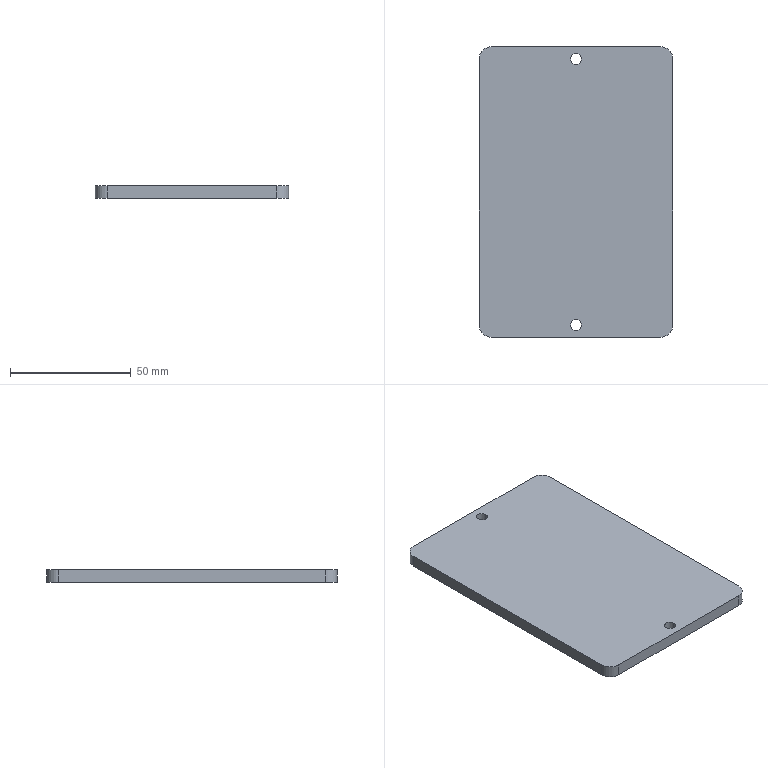Part | STEP file | Acrylic cover plate | 1 solid | 14 faces | box 80 x 120 x 5 mm | volume 47734 mm3 | cylinder 8 | plane 6 | commonest cylinder face diameters 4.5 x4 10 x4
STEP:
#1=CARTESIAN_POINT('',(0.,0.,0.));
#2=DIRECTION('',(0.,0.,1.));
#3=DIRECTION('',(1.,0.,0.));
#4=AXIS2_PLACEMENT_3D('',#1,#2,#3);
#5=CARTESIAN_POINT('',(-2.25,-55.,5.));
#6=VERTEX_POINT('',#5);
#7=CARTESIAN_POINT('',(-2.25,-55.,0.));
#8=VERTEX_POINT('',#7);
#9=CARTESIAN_POINT('',(-2.25,-55.,5.));
#10=DIRECTION('',(0.,0.,-1.));
#11=VECTOR('',#10,1.);
#12=LINE('',#9,#11);
#13=CARTESIAN_POINT('',(0.,-55.,5.));
#14=DIRECTION('',(0.,0.,-1.));
#15=DIRECTION('',(-1.,0.,0.));
#16=AXIS2_PLACEMENT_3D('',#13,#14,#15);
#17=CYLINDRICAL_SURFACE('',#16,2.25);
#18=CARTESIAN_POINT('',(6.283,0.));
#19=DIRECTION('',(0.,1.));
#20=VECTOR('',#19,1.);
#21=LINE('',#18,#20);
#22=(GEOMETRIC_REPRESENTATION_CONTEXT(2)PARAMETRIC_REPRESENTATION_CONTEXT()REPRESENTATION_CONTEXT('',''));
#23=DEFINITIONAL_REPRESENTATION('',(#21),#22);
#24=PCURVE('',#17,#23);
#25=CARTESIAN_POINT('',(0.,-55.,5.));
#26=DIRECTION('',(0.,0.,-1.));
#27=DIRECTION('',(-1.,0.,0.));
#28=AXIS2_PLACEMENT_3D('',#25,#26,#27);
#29=CYLINDRICAL_SURFACE('',#28,2.25);
#30=CARTESIAN_POINT('',(0.,0.));
#31=DIRECTION('',(0.,1.));
#32=VECTOR('',#31,1.);
#33=LINE('',#30,#32);
#34=(GEOMETRIC_REPRESENTATION_CONTEXT(2)PARAMETRIC_REPRESENTATION_CONTEXT()REPRESENTATION_CONTEXT('',''));
#35=DEFINITIONAL_REPRESENTATION('',(#33),#34);
#36=PCURVE('',#29,#35);
#37=SURFACE_CURVE('',#12,(#24,#36),.PCURVE_S1.);
#38=EDGE_CURVE('',#6,#8,#37,.T.);
#39=ORIENTED_EDGE('',*,*,#38,.T.);
#40=CARTESIAN_POINT('',(2.25,-55.,0.));
#41=VERTEX_POINT('',#40);
#42=CARTESIAN_POINT('',(0.,-55.,0.));
#43=DIRECTION('',(0.,0.,1.));
#44=DIRECTION('',(-1.,0.,0.));
#45=AXIS2_PLACEMENT_3D('',#42,#43,#44);
#46=CIRCLE('',#45,2.25);
#47=CARTESIAN_POINT('',(6.283,5.));
#48=DIRECTION('',(-1.,0.));
#49=VECTOR('',#48,1.);
#50=LINE('',#47,#49);
#51=(GEOMETRIC_REPRESENTATION_CONTEXT(2)PARAMETRIC_REPRESENTATION_CONTEXT()REPRESENTATION_CONTEXT('',''));
#52=DEFINITIONAL_REPRESENTATION('',(#50),#51);
#53=PCURVE('',#17,#52);
#54=CARTESIAN_POINT('',(35.,55.,0.));
#55=DIRECTION('',(0.,0.,-1.));
#56=DIRECTION('',(-1.,0.,0.));
#57=AXIS2_PLACEMENT_3D('',#54,#55,#56);
#58=PLANE('',#57);
#59=CARTESIAN_POINT('',(37.25,-110.));
#60=CARTESIAN_POINT('',(37.25,-113.897));
#61=CARTESIAN_POINT('',(33.875,-111.949));
#62=CARTESIAN_POINT('',(30.5,-110.));
#63=CARTESIAN_POINT('',(33.875,-108.051));
#64=CARTESIAN_POINT('',(37.25,-106.103));
#65=CARTESIAN_POINT('',(37.25,-110.));
#66=(BOUNDED_CURVE()B_SPLINE_CURVE(2,(#59,#60,#61,#62,#63,#64,#65),.UNSPECIFIED.,.T.,.F.)B_SPLINE_CURVE_WITH_KNOTS((1,2,2,2,2,1),(-2.094,0.,2.094,4.189,6.283,8.378),.UNSPECIFIED.)CURVE()GEOMETRIC_REPRESENTATION_ITEM()RATIONAL_B_SPLINE_CURVE((1.,0.5,1.,0.5,1.,0.5,1.))REPRESENTATION_ITEM(''));
#67=(GEOMETRIC_REPRESENTATION_CONTEXT(2)PARAMETRIC_REPRESENTATION_CONTEXT()REPRESENTATION_CONTEXT('',''));
#68=DEFINITIONAL_REPRESENTATION('',(#66),#67);
#69=PCURVE('',#58,#68);
#70=SURFACE_CURVE('',#46,(#53,#69),.PCURVE_S1.);
#71=EDGE_CURVE('',#8,#41,#70,.T.);
#72=ORIENTED_EDGE('',*,*,#71,.T.);
#73=CARTESIAN_POINT('',(2.25,-55.,5.));
#74=VERTEX_POINT('',#73);
#75=CARTESIAN_POINT('',(2.25,-55.,5.));
#76=DIRECTION('',(0.,0.,-1.));
#77=VECTOR('',#76,1.);
#78=LINE('',#75,#77);
#79=CARTESIAN_POINT('',(3.142,0.));
#80=DIRECTION('',(0.,1.));
#81=VECTOR('',#80,1.);
#82=LINE('',#79,#81);
#83=(GEOMETRIC_REPRESENTATION_CONTEXT(2)PARAMETRIC_REPRESENTATION_CONTEXT()REPRESENTATION_CONTEXT('',''));
#84=DEFINITIONAL_REPRESENTATION('',(#82),#83);
#85=PCURVE('',#17,#84);
#86=CARTESIAN_POINT('',(3.142,0.));
#87=DIRECTION('',(0.,1.));
#88=VECTOR('',#87,1.);
#89=LINE('',#86,#88);
#90=(GEOMETRIC_REPRESENTATION_CONTEXT(2)PARAMETRIC_REPRESENTATION_CONTEXT()REPRESENTATION_CONTEXT('',''));
#91=DEFINITIONAL_REPRESENTATION('',(#89),#90);
#92=PCURVE('',#29,#91);
#93=SURFACE_CURVE('',#78,(#85,#92),.PCURVE_S1.);
#94=EDGE_CURVE('',#74,#41,#93,.T.);
#95=ORIENTED_EDGE('',*,*,#94,.F.);
#96=CARTESIAN_POINT('',(0.,-55.,5.));
#97=DIRECTION('',(0.,0.,1.));
#98=DIRECTION('',(-1.,0.,0.));
#99=AXIS2_PLACEMENT_3D('',#96,#97,#98);
#100=CIRCLE('',#99,2.25);
#101=CARTESIAN_POINT('',(6.283,0.));
#102=DIRECTION('',(-1.,0.));
#103=VECTOR('',#102,1.);
#104=LINE('',#101,#103);
#105=(GEOMETRIC_REPRESENTATION_CONTEXT(2)PARAMETRIC_REPRESENTATION_CONTEXT()REPRESENTATION_CONTEXT('',''));
#106=DEFINITIONAL_REPRESENTATION('',(#104),#105);
#107=PCURVE('',#17,#106);
#108=CARTESIAN_POINT('',(35.,55.,5.));
#109=DIRECTION('',(0.,0.,-1.));
#110=DIRECTION('',(-1.,0.,0.));
#111=AXIS2_PLACEMENT_3D('',#108,#109,#110);
#112=PLANE('',#111);
#113=CARTESIAN_POINT('',(37.25,-110.));
#114=CARTESIAN_POINT('',(37.25,-113.897));
#115=CARTESIAN_POINT('',(33.875,-111.949));
#116=CARTESIAN_POINT('',(30.5,-110.));
#117=CARTESIAN_POINT('',(33.875,-108.051));
#118=CARTESIAN_POINT('',(37.25,-106.103));
#119=CARTESIAN_POINT('',(37.25,-110.));
#120=(BOUNDED_CURVE()B_SPLINE_CURVE(2,(#113,#114,#115,#116,#117,#118,#119),.UNSPECIFIED.,.T.,.F.)B_SPLINE_CURVE_WITH_KNOTS((1,2,2,2,2,1),(-2.094,0.,2.094,4.189,6.283,8.378),.UNSPECIFIED.)CURVE()GEOMETRIC_REPRESENTATION_ITEM()RATIONAL_B_SPLINE_CURVE((1.,0.5,1.,0.5,1.,0.5,1.))REPRESENTATION_ITEM(''));
#121=(GEOMETRIC_REPRESENTATION_CONTEXT(2)PARAMETRIC_REPRESENTATION_CONTEXT()REPRESENTATION_CONTEXT('',''));
#122=DEFINITIONAL_REPRESENTATION('',(#120),#121);
#123=PCURVE('',#112,#122);
#124=SURFACE_CURVE('',#100,(#107,#123),.PCURVE_S1.);
#125=EDGE_CURVE('',#6,#74,#124,.T.);
#126=ORIENTED_EDGE('',*,*,#125,.F.);
#127=EDGE_LOOP('',(#39,#72,#95,#126));
#128=FACE_BOUND('',#127,.F.);
#129=ADVANCED_FACE('',(#128),#17,.F.);
#130=CARTESIAN_POINT('',(-2.25,55.,5.));
#131=VERTEX_POINT('',#130);
#132=CARTESIAN_POINT('',(-2.25,55.,0.));
#133=VERTEX_POINT('',#132);
#134=CARTESIAN_POINT('',(-2.25,55.,5.));
#135=DIRECTION('',(0.,0.,-1.));
#136=VECTOR('',#135,1.);
#137=LINE('',#134,#136);
#138=CARTESIAN_POINT('',(0.,55.,5.));
#139=DIRECTION('',(0.,0.,-1.));
#140=DIRECTION('',(-1.,0.,0.));
#141=AXIS2_PLACEMENT_3D('',#138,#139,#140);
#142=CYLINDRICAL_SURFACE('',#141,2.25);
#143=CARTESIAN_POINT('',(6.283,0.));
#144=DIRECTION('',(0.,1.));
#145=VECTOR('',#144,1.);
#146=LINE('',#143,#145);
#147=(GEOMETRIC_REPRESENTATION_CONTEXT(2)PARAMETRIC_REPRESENTATION_CONTEXT()REPRESENTATION_CONTEXT('',''));
#148=DEFINITIONAL_REPRESENTATION('',(#146),#147);
#149=PCURVE('',#142,#148);
#150=CARTESIAN_POINT('',(0.,55.,5.));
#151=DIRECTION('',(0.,0.,-1.));
#152=DIRECTION('',(-1.,0.,0.));
#153=AXIS2_PLACEMENT_3D('',#150,#151,#152);
#154=CYLINDRICAL_SURFACE('',#153,2.25);
#155=CARTESIAN_POINT('',(0.,0.));
#156=DIRECTION('',(0.,1.));
#157=VECTOR('',#156,1.);
#158=LINE('',#155,#157);
#159=(GEOMETRIC_REPRESENTATION_CONTEXT(2)PARAMETRIC_REPRESENTATION_CONTEXT()REPRESENTATION_CONTEXT('',''));
#160=DEFINITIONAL_REPRESENTATION('',(#158),#159);
#161=PCURVE('',#154,#160);
#162=SURFACE_CURVE('',#137,(#149,#161),.PCURVE_S1.);
#163=EDGE_CURVE('',#131,#133,#162,.T.);
#164=ORIENTED_EDGE('',*,*,#163,.T.);
#165=CARTESIAN_POINT('',(2.25,55.,0.));
#166=VERTEX_POINT('',#165);
#167=CARTESIAN_POINT('',(0.,55.,0.));
#168=DIRECTION('',(0.,0.,1.));
#169=DIRECTION('',(-1.,0.,0.));
#170=AXIS2_PLACEMENT_3D('',#167,#168,#169);
#171=CIRCLE('',#170,2.25);
#172=CARTESIAN_POINT('',(6.283,5.));
#173=DIRECTION('',(-1.,0.));
#174=VECTOR('',#173,1.);
#175=LINE('',#172,#174);
#176=(GEOMETRIC_REPRESENTATION_CONTEXT(2)PARAMETRIC_REPRESENTATION_CONTEXT()REPRESENTATION_CONTEXT('',''));
#177=DEFINITIONAL_REPRESENTATION('',(#175),#176);
#178=PCURVE('',#142,#177);
#179=CARTESIAN_POINT('',(37.25,0.));
#180=CARTESIAN_POINT('',(37.25,-3.897));
#181=CARTESIAN_POINT('',(33.875,-1.949));
#182=CARTESIAN_POINT('',(30.5,0.));
#183=CARTESIAN_POINT('',(33.875,1.949));
#184=CARTESIAN_POINT('',(37.25,3.897));
#185=CARTESIAN_POINT('',(37.25,0.));
#186=(BOUNDED_CURVE()B_SPLINE_CURVE(2,(#179,#180,#181,#182,#183,#184,#185),.UNSPECIFIED.,.T.,.F.)B_SPLINE_CURVE_WITH_KNOTS((1,2,2,2,2,1),(-2.094,0.,2.094,4.189,6.283,8.378),.UNSPECIFIED.)CURVE()GEOMETRIC_REPRESENTATION_ITEM()RATIONAL_B_SPLINE_CURVE((1.,0.5,1.,0.5,1.,0.5,1.))REPRESENTATION_ITEM(''));
#187=(GEOMETRIC_REPRESENTATION_CONTEXT(2)PARAMETRIC_REPRESENTATION_CONTEXT()REPRESENTATION_CONTEXT('',''));
#188=DEFINITIONAL_REPRESENTATION('',(#186),#187);
#189=PCURVE('',#58,#188);
#190=SURFACE_CURVE('',#171,(#178,#189),.PCURVE_S1.);
#191=EDGE_CURVE('',#133,#166,#190,.T.);
#192=ORIENTED_EDGE('',*,*,#191,.T.);
#193=CARTESIAN_POINT('',(2.25,55.,5.));
#194=VERTEX_POINT('',#193);
#195=CARTESIAN_POINT('',(2.25,55.,5.));
#196=DIRECTION('',(0.,0.,-1.));
#197=VECTOR('',#196,1.);
#198=LINE('',#195,#197);
#199=CARTESIAN_POINT('',(3.142,0.));
#200=DIRECTION('',(0.,1.));
#201=VECTOR('',#200,1.);
#202=LINE('',#199,#201);
#203=(GEOMETRIC_REPRESENTATION_CONTEXT(2)PARAMETRIC_REPRESENTATION_CONTEXT()REPRESENTATION_CONTEXT('',''));
#204=DEFINITIONAL_REPRESENTATION('',(#202),#203);
#205=PCURVE('',#142,#204);
#206=CARTESIAN_POINT('',(3.142,0.));
#207=DIRECTION('',(0.,1.));
#208=VECTOR('',#207,1.);
#209=LINE('',#206,#208);
#210=(GEOMETRIC_REPRESENTATION_CONTEXT(2)PARAMETRIC_REPRESENTATION_CONTEXT()REPRESENTATION_CONTEXT('',''));
#211=DEFINITIONAL_REPRESENTATION('',(#209),#210);
#212=PCURVE('',#154,#211);
#213=SURFACE_CURVE('',#198,(#205,#212),.PCURVE_S1.);
#214=EDGE_CURVE('',#194,#166,#213,.T.);
#215=ORIENTED_EDGE('',*,*,#214,.F.);
#216=CARTESIAN_POINT('',(0.,55.,5.));
#217=DIRECTION('',(0.,0.,1.));
#218=DIRECTION('',(-1.,0.,0.));
#219=AXIS2_PLACEMENT_3D('',#216,#217,#218);
#220=CIRCLE('',#219,2.25);
#221=CARTESIAN_POINT('',(6.283,0.));
#222=DIRECTION('',(-1.,0.));
#223=VECTOR('',#222,1.);
#224=LINE('',#221,#223);
#225=(GEOMETRIC_REPRESENTATION_CONTEXT(2)PARAMETRIC_REPRESENTATION_CONTEXT()REPRESENTATION_CONTEXT('',''));
#226=DEFINITIONAL_REPRESENTATION('',(#224),#225);
#227=PCURVE('',#142,#226);
#228=CARTESIAN_POINT('',(37.25,0.));
#229=CARTESIAN_POINT('',(37.25,-3.897));
#230=CARTESIAN_POINT('',(33.875,-1.949));
#231=CARTESIAN_POINT('',(30.5,0.));
#232=CARTESIAN_POINT('',(33.875,1.949));
#233=CARTESIAN_POINT('',(37.25,3.897));
#234=CARTESIAN_POINT('',(37.25,0.));
#235=(BOUNDED_CURVE()B_SPLINE_CURVE(2,(#228,#229,#230,#231,#232,#233,#234),.UNSPECIFIED.,.T.,.F.)B_SPLINE_CURVE_WITH_KNOTS((1,2,2,2,2,1),(-2.094,0.,2.094,4.189,6.283,8.378),.UNSPECIFIED.)CURVE()GEOMETRIC_REPRESENTATION_ITEM()RATIONAL_B_SPLINE_CURVE((1.,0.5,1.,0.5,1.,0.5,1.))REPRESENTATION_ITEM(''));
#236=(GEOMETRIC_REPRESENTATION_CONTEXT(2)PARAMETRIC_REPRESENTATION_CONTEXT()REPRESENTATION_CONTEXT('',''));
#237=DEFINITIONAL_REPRESENTATION('',(#235),#236);
#238=PCURVE('',#112,#237);
#239=SURFACE_CURVE('',#220,(#227,#238),.PCURVE_S1.);
#240=EDGE_CURVE('',#131,#194,#239,.T.);
#241=ORIENTED_EDGE('',*,*,#240,.F.);
#242=EDGE_LOOP('',(#164,#192,#215,#241));
#243=FACE_BOUND('',#242,.F.);
#244=ADVANCED_FACE('',(#243),#142,.F.);
#245=ORIENTED_EDGE('',*,*,#125,.F.);
#246=CARTESIAN_POINT('',(0.,-55.,5.));
#247=DIRECTION('',(0.,0.,1.));
#248=DIRECTION('',(-1.,0.,0.));
#249=AXIS2_PLACEMENT_3D('',#246,#247,#248);
#250=CIRCLE('',#249,2.25);
#251=CARTESIAN_POINT('',(37.25,-110.));
#252=CARTESIAN_POINT('',(37.25,-113.897));
#253=CARTESIAN_POINT('',(33.875,-111.949));
#254=CARTESIAN_POINT('',(30.5,-110.));
#255=CARTESIAN_POINT('',(33.875,-108.051));
#256=CARTESIAN_POINT('',(37.25,-106.103));
#257=CARTESIAN_POINT('',(37.25,-110.));
#258=(BOUNDED_CURVE()B_SPLINE_CURVE(2,(#251,#252,#253,#254,#255,#256,#257),.UNSPECIFIED.,.T.,.F.)B_SPLINE_CURVE_WITH_KNOTS((1,2,2,2,2,1),(-2.094,0.,2.094,4.189,6.283,8.378),.UNSPECIFIED.)CURVE()GEOMETRIC_REPRESENTATION_ITEM()RATIONAL_B_SPLINE_CURVE((1.,0.5,1.,0.5,1.,0.5,1.))REPRESENTATION_ITEM(''));
#259=(GEOMETRIC_REPRESENTATION_CONTEXT(2)PARAMETRIC_REPRESENTATION_CONTEXT()REPRESENTATION_CONTEXT('',''));
#260=DEFINITIONAL_REPRESENTATION('',(#258),#259);
#261=PCURVE('',#112,#260);
#262=CARTESIAN_POINT('',(6.283,0.));
#263=DIRECTION('',(-1.,0.));
#264=VECTOR('',#263,1.);
#265=LINE('',#262,#264);
#266=(GEOMETRIC_REPRESENTATION_CONTEXT(2)PARAMETRIC_REPRESENTATION_CONTEXT()REPRESENTATION_CONTEXT('',''));
#267=DEFINITIONAL_REPRESENTATION('',(#265),#266);
#268=PCURVE('',#29,#267);
#269=SURFACE_CURVE('',#250,(#261,#268),.PCURVE_S1.);
#270=EDGE_CURVE('',#74,#6,#269,.T.);
#271=ORIENTED_EDGE('',*,*,#270,.F.);
#272=EDGE_LOOP('',(#245,#271));
#273=FACE_BOUND('',#272,.T.);
#274=CARTESIAN_POINT('',(-35.,60.,5.));
#275=VERTEX_POINT('',#274);
#276=CARTESIAN_POINT('',(35.,60.,5.));
#277=VERTEX_POINT('',#276);
#278=CARTESIAN_POINT('',(35.,60.,5.));
#279=DIRECTION('',(1.,0.,0.));
#280=VECTOR('',#279,1.);
#281=LINE('',#278,#280);
#282=CARTESIAN_POINT('',(0.,5.));
#283=DIRECTION('',(-1.,0.));
#284=VECTOR('',#283,1.);
#285=LINE('',#282,#284);
#286=(GEOMETRIC_REPRESENTATION_CONTEXT(2)PARAMETRIC_REPRESENTATION_CONTEXT()REPRESENTATION_CONTEXT('',''));
#287=DEFINITIONAL_REPRESENTATION('',(#285),#286);
#288=PCURVE('',#112,#287);
#289=CARTESIAN_POINT('',(-35.,60.,5.));
#290=DIRECTION('',(0.,-1.,0.));
#291=DIRECTION('',(0.,0.,-1.));
#292=AXIS2_PLACEMENT_3D('',#289,#290,#291);
#293=PLANE('',#292);
#294=CARTESIAN_POINT('',(0.,70.));
#295=DIRECTION('',(0.,1.));
#296=VECTOR('',#295,1.);
#297=LINE('',#294,#296);
#298=(GEOMETRIC_REPRESENTATION_CONTEXT(2)PARAMETRIC_REPRESENTATION_CONTEXT()REPRESENTATION_CONTEXT('',''));
#299=DEFINITIONAL_REPRESENTATION('',(#297),#298);
#300=PCURVE('',#293,#299);
#301=SURFACE_CURVE('',#281,(#288,#300),.PCURVE_S1.);
#302=EDGE_CURVE('',#275,#277,#301,.T.);
#303=ORIENTED_EDGE('',*,*,#302,.F.);
#304=CARTESIAN_POINT('',(-40.,55.,5.));
#305=VERTEX_POINT('',#304);
#306=CARTESIAN_POINT('',(-35.,55.,5.));
#307=DIRECTION('',(0.,0.,-1.));
#308=DIRECTION('',(-1.,0.,0.));
#309=AXIS2_PLACEMENT_3D('',#306,#307,#308);
#310=CIRCLE('',#309,5.);
#311=CARTESIAN_POINT('',(70.,0.));
#312=DIRECTION('',(1.,0.));
#313=AXIS2_PLACEMENT_2D('',#311,#312);
#314=CIRCLE('',#313,5.);
#315=(GEOMETRIC_REPRESENTATION_CONTEXT(2)PARAMETRIC_REPRESENTATION_CONTEXT()REPRESENTATION_CONTEXT('',''));
#316=DEFINITIONAL_REPRESENTATION('',(#314),#315);
#317=PCURVE('',#112,#316);
#318=CARTESIAN_POINT('',(-35.,55.,5.));
#319=DIRECTION('',(0.,0.,-1.));
#320=DIRECTION('',(-1.,0.,0.));
#321=AXIS2_PLACEMENT_3D('',#318,#319,#320);
#322=CYLINDRICAL_SURFACE('',#321,5.);
#323=CARTESIAN_POINT('',(0.,0.));
#324=DIRECTION('',(1.,0.));
#325=VECTOR('',#324,1.);
#326=LINE('',#323,#325);
#327=(GEOMETRIC_REPRESENTATION_CONTEXT(2)PARAMETRIC_REPRESENTATION_CONTEXT()REPRESENTATION_CONTEXT('',''));
#328=DEFINITIONAL_REPRESENTATION('',(#326),#327);
#329=PCURVE('',#322,#328);
#330=SURFACE_CURVE('',#310,(#317,#329),.PCURVE_S1.);
#331=EDGE_CURVE('',#305,#275,#330,.T.);
#332=ORIENTED_EDGE('',*,*,#331,.F.);
#333=CARTESIAN_POINT('',(-40.,-55.,5.));
#334=VERTEX_POINT('',#333);
#335=CARTESIAN_POINT('',(-40.,55.,5.));
#336=DIRECTION('',(0.,1.,0.));
#337=VECTOR('',#336,1.);
#338=LINE('',#335,#337);
#339=CARTESIAN_POINT('',(75.,0.));
#340=DIRECTION('',(0.,1.));
#341=VECTOR('',#340,1.);
#342=LINE('',#339,#341);
#343=(GEOMETRIC_REPRESENTATION_CONTEXT(2)PARAMETRIC_REPRESENTATION_CONTEXT()REPRESENTATION_CONTEXT('',''));
#344=DEFINITIONAL_REPRESENTATION('',(#342),#343);
#345=PCURVE('',#112,#344);
#346=CARTESIAN_POINT('',(-40.,55.,5.));
#347=DIRECTION('',(1.,0.,0.));
#348=DIRECTION('',(0.,1.,0.));
#349=AXIS2_PLACEMENT_3D('',#346,#347,#348);
#350=PLANE('',#349);
#351=CARTESIAN_POINT('',(0.,0.));
#352=DIRECTION('',(1.,0.));
#353=VECTOR('',#352,1.);
#354=LINE('',#351,#353);
#355=(GEOMETRIC_REPRESENTATION_CONTEXT(2)PARAMETRIC_REPRESENTATION_CONTEXT()REPRESENTATION_CONTEXT('',''));
#356=DEFINITIONAL_REPRESENTATION('',(#354),#355);
#357=PCURVE('',#350,#356);
#358=SURFACE_CURVE('',#338,(#345,#357),.PCURVE_S1.);
#359=EDGE_CURVE('',#334,#305,#358,.T.);
#360=ORIENTED_EDGE('',*,*,#359,.F.);
#361=CARTESIAN_POINT('',(-35.,-60.,5.));
#362=VERTEX_POINT('',#361);
#363=CARTESIAN_POINT('',(-35.,-55.,5.));
#364=DIRECTION('',(0.,0.,-1.));
#365=DIRECTION('',(-1.,0.,0.));
#366=AXIS2_PLACEMENT_3D('',#363,#364,#365);
#367=CIRCLE('',#366,5.);
#368=CARTESIAN_POINT('',(70.,-110.));
#369=DIRECTION('',(1.,0.));
#370=AXIS2_PLACEMENT_2D('',#368,#369);
#371=CIRCLE('',#370,5.);
#372=(GEOMETRIC_REPRESENTATION_CONTEXT(2)PARAMETRIC_REPRESENTATION_CONTEXT()REPRESENTATION_CONTEXT('',''));
#373=DEFINITIONAL_REPRESENTATION('',(#371),#372);
#374=PCURVE('',#112,#373);
#375=CARTESIAN_POINT('',(-35.,-55.,5.));
#376=DIRECTION('',(0.,0.,-1.));
#377=DIRECTION('',(-1.,0.,0.));
#378=AXIS2_PLACEMENT_3D('',#375,#376,#377);
#379=CYLINDRICAL_SURFACE('',#378,5.);
#380=CARTESIAN_POINT('',(0.,0.));
#381=DIRECTION('',(1.,0.));
#382=VECTOR('',#381,1.);
#383=LINE('',#380,#382);
#384=(GEOMETRIC_REPRESENTATION_CONTEXT(2)PARAMETRIC_REPRESENTATION_CONTEXT()REPRESENTATION_CONTEXT('',''));
#385=DEFINITIONAL_REPRESENTATION('',(#383),#384);
#386=PCURVE('',#379,#385);
#387=SURFACE_CURVE('',#367,(#374,#386),.PCURVE_S1.);
#388=EDGE_CURVE('',#362,#334,#387,.T.);
#389=ORIENTED_EDGE('',*,*,#388,.F.);
#390=CARTESIAN_POINT('',(35.,-60.,5.));
#391=VERTEX_POINT('',#390);
#392=CARTESIAN_POINT('',(35.,-60.,5.));
#393=DIRECTION('',(-1.,0.,0.));
#394=VECTOR('',#393,1.);
#395=LINE('',#392,#394);
#396=CARTESIAN_POINT('',(0.,-115.));
#397=DIRECTION('',(1.,0.));
#398=VECTOR('',#397,1.);
#399=LINE('',#396,#398);
#400=(GEOMETRIC_REPRESENTATION_CONTEXT(2)PARAMETRIC_REPRESENTATION_CONTEXT()REPRESENTATION_CONTEXT('',''));
#401=DEFINITIONAL_REPRESENTATION('',(#399),#400);
#402=PCURVE('',#112,#401);
#403=CARTESIAN_POINT('',(-35.,-60.,5.));
#404=DIRECTION('',(0.,1.,0.));
#405=DIRECTION('',(0.,0.,1.));
#406=AXIS2_PLACEMENT_3D('',#403,#404,#405);
#407=PLANE('',#406);
#408=CARTESIAN_POINT('',(0.,70.));
#409=DIRECTION('',(0.,-1.));
#410=VECTOR('',#409,1.);
#411=LINE('',#408,#410);
#412=(GEOMETRIC_REPRESENTATION_CONTEXT(2)PARAMETRIC_REPRESENTATION_CONTEXT()REPRESENTATION_CONTEXT('',''));
#413=DEFINITIONAL_REPRESENTATION('',(#411),#412);
#414=PCURVE('',#407,#413);
#415=SURFACE_CURVE('',#395,(#402,#414),.PCURVE_S1.);
#416=EDGE_CURVE('',#391,#362,#415,.T.);
#417=ORIENTED_EDGE('',*,*,#416,.F.);
#418=CARTESIAN_POINT('',(40.,-55.,5.));
#419=VERTEX_POINT('',#418);
#420=CARTESIAN_POINT('',(35.,-55.,5.));
#421=DIRECTION('',(0.,0.,-1.));
#422=DIRECTION('',(-1.,0.,0.));
#423=AXIS2_PLACEMENT_3D('',#420,#421,#422);
#424=CIRCLE('',#423,5.);
#425=CARTESIAN_POINT('',(0.,-110.));
#426=DIRECTION('',(1.,0.));
#427=AXIS2_PLACEMENT_2D('',#425,#426);
#428=CIRCLE('',#427,5.);
#429=(GEOMETRIC_REPRESENTATION_CONTEXT(2)PARAMETRIC_REPRESENTATION_CONTEXT()REPRESENTATION_CONTEXT('',''));
#430=DEFINITIONAL_REPRESENTATION('',(#428),#429);
#431=PCURVE('',#112,#430);
#432=CARTESIAN_POINT('',(35.,-55.,5.));
#433=DIRECTION('',(0.,0.,-1.));
#434=DIRECTION('',(-1.,0.,0.));
#435=AXIS2_PLACEMENT_3D('',#432,#433,#434);
#436=CYLINDRICAL_SURFACE('',#435,5.);
#437=CARTESIAN_POINT('',(0.,0.));
#438=DIRECTION('',(1.,0.));
#439=VECTOR('',#438,1.);
#440=LINE('',#437,#439);
#441=(GEOMETRIC_REPRESENTATION_CONTEXT(2)PARAMETRIC_REPRESENTATION_CONTEXT()REPRESENTATION_CONTEXT('',''));
#442=DEFINITIONAL_REPRESENTATION('',(#440),#441);
#443=PCURVE('',#436,#442);
#444=SURFACE_CURVE('',#424,(#431,#443),.PCURVE_S1.);
#445=EDGE_CURVE('',#419,#391,#444,.T.);
#446=ORIENTED_EDGE('',*,*,#445,.F.);
#447=CARTESIAN_POINT('',(40.,55.,5.));
#448=VERTEX_POINT('',#447);
#449=CARTESIAN_POINT('',(40.,55.,5.));
#450=DIRECTION('',(0.,-1.,0.));
#451=VECTOR('',#450,1.);
#452=LINE('',#449,#451);
#453=CARTESIAN_POINT('',(-5.,0.));
#454=DIRECTION('',(0.,-1.));
#455=VECTOR('',#454,1.);
#456=LINE('',#453,#455);
#457=(GEOMETRIC_REPRESENTATION_CONTEXT(2)PARAMETRIC_REPRESENTATION_CONTEXT()REPRESENTATION_CONTEXT('',''));
#458=DEFINITIONAL_REPRESENTATION('',(#456),#457);
#459=PCURVE('',#112,#458);
#460=CARTESIAN_POINT('',(40.,55.,5.));
#461=DIRECTION('',(-1.,0.,0.));
#462=DIRECTION('',(0.,-1.,0.));
#463=AXIS2_PLACEMENT_3D('',#460,#461,#462);
#464=PLANE('',#463);
#465=CARTESIAN_POINT('',(0.,0.));
#466=DIRECTION('',(1.,0.));
#467=VECTOR('',#466,1.);
#468=LINE('',#465,#467);
#469=(GEOMETRIC_REPRESENTATION_CONTEXT(2)PARAMETRIC_REPRESENTATION_CONTEXT()REPRESENTATION_CONTEXT('',''));
#470=DEFINITIONAL_REPRESENTATION('',(#468),#469);
#471=PCURVE('',#464,#470);
#472=SURFACE_CURVE('',#452,(#459,#471),.PCURVE_S1.);
#473=EDGE_CURVE('',#448,#419,#472,.T.);
#474=ORIENTED_EDGE('',*,*,#473,.F.);
#475=CARTESIAN_POINT('',(35.,55.,5.));
#476=DIRECTION('',(0.,0.,-1.));
#477=DIRECTION('',(-1.,0.,0.));
#478=AXIS2_PLACEMENT_3D('',#475,#476,#477);
#479=CIRCLE('',#478,5.);
#480=CARTESIAN_POINT('',(0.,0.));
#481=DIRECTION('',(1.,0.));
#482=AXIS2_PLACEMENT_2D('',#480,#481);
#483=CIRCLE('',#482,5.);
#484=(GEOMETRIC_REPRESENTATION_CONTEXT(2)PARAMETRIC_REPRESENTATION_CONTEXT()REPRESENTATION_CONTEXT('',''));
#485=DEFINITIONAL_REPRESENTATION('',(#483),#484);
#486=PCURVE('',#112,#485);
#487=CARTESIAN_POINT('',(35.,55.,5.));
#488=DIRECTION('',(0.,0.,-1.));
#489=DIRECTION('',(-1.,0.,0.));
#490=AXIS2_PLACEMENT_3D('',#487,#488,#489);
#491=CYLINDRICAL_SURFACE('',#490,5.);
#492=CARTESIAN_POINT('',(0.,0.));
#493=DIRECTION('',(1.,0.));
#494=VECTOR('',#493,1.);
#495=LINE('',#492,#494);
#496=(GEOMETRIC_REPRESENTATION_CONTEXT(2)PARAMETRIC_REPRESENTATION_CONTEXT()REPRESENTATION_CONTEXT('',''));
#497=DEFINITIONAL_REPRESENTATION('',(#495),#496);
#498=PCURVE('',#491,#497);
#499=SURFACE_CURVE('',#479,(#486,#498),.PCURVE_S1.);
#500=EDGE_CURVE('',#277,#448,#499,.T.);
#501=ORIENTED_EDGE('',*,*,#500,.F.);
#502=EDGE_LOOP('',(#303,#332,#360,#389,#417,#446,#474,#501));
#503=FACE_BOUND('',#502,.T.);
#504=ORIENTED_EDGE('',*,*,#240,.F.);
#505=CARTESIAN_POINT('',(0.,55.,5.));
#506=DIRECTION('',(0.,0.,1.));
#507=DIRECTION('',(-1.,0.,0.));
#508=AXIS2_PLACEMENT_3D('',#505,#506,#507);
#509=CIRCLE('',#508,2.25);
#510=CARTESIAN_POINT('',(37.25,0.));
#511=CARTESIAN_POINT('',(37.25,-3.897));
#512=CARTESIAN_POINT('',(33.875,-1.949));
#513=CARTESIAN_POINT('',(30.5,0.));
#514=CARTESIAN_POINT('',(33.875,1.949));
#515=CARTESIAN_POINT('',(37.25,3.897));
#516=CARTESIAN_POINT('',(37.25,0.));
#517=(BOUNDED_CURVE()B_SPLINE_CURVE(2,(#510,#511,#512,#513,#514,#515,#516),.UNSPECIFIED.,.T.,.F.)B_SPLINE_CURVE_WITH_KNOTS((1,2,2,2,2,1),(-2.094,0.,2.094,4.189,6.283,8.378),.UNSPECIFIED.)CURVE()GEOMETRIC_REPRESENTATION_ITEM()RATIONAL_B_SPLINE_CURVE((1.,0.5,1.,0.5,1.,0.5,1.))REPRESENTATION_ITEM(''));
#518=(GEOMETRIC_REPRESENTATION_CONTEXT(2)PARAMETRIC_REPRESENTATION_CONTEXT()REPRESENTATION_CONTEXT('',''));
#519=DEFINITIONAL_REPRESENTATION('',(#517),#518);
#520=PCURVE('',#112,#519);
#521=CARTESIAN_POINT('',(6.283,0.));
#522=DIRECTION('',(-1.,0.));
#523=VECTOR('',#522,1.);
#524=LINE('',#521,#523);
#525=(GEOMETRIC_REPRESENTATION_CONTEXT(2)PARAMETRIC_REPRESENTATION_CONTEXT()REPRESENTATION_CONTEXT('',''));
#526=DEFINITIONAL_REPRESENTATION('',(#524),#525);
#527=PCURVE('',#154,#526);
#528=SURFACE_CURVE('',#509,(#520,#527),.PCURVE_S1.);
#529=EDGE_CURVE('',#194,#131,#528,.T.);
#530=ORIENTED_EDGE('',*,*,#529,.F.);
#531=EDGE_LOOP('',(#504,#530));
#532=FACE_BOUND('',#531,.T.);
#533=ADVANCED_FACE('',(#273,#503,#532),#112,.F.);
#534=CARTESIAN_POINT('',(0.,-55.,0.));
#535=DIRECTION('',(0.,0.,1.));
#536=DIRECTION('',(-1.,0.,0.));
#537=AXIS2_PLACEMENT_3D('',#534,#535,#536);
#538=CIRCLE('',#537,2.25);
#539=CARTESIAN_POINT('',(6.283,5.));
#540=DIRECTION('',(-1.,0.));
#541=VECTOR('',#540,1.);
#542=LINE('',#539,#541);
#543=(GEOMETRIC_REPRESENTATION_CONTEXT(2)PARAMETRIC_REPRESENTATION_CONTEXT()REPRESENTATION_CONTEXT('',''));
#544=DEFINITIONAL_REPRESENTATION('',(#542),#543);
#545=PCURVE('',#29,#544);
#546=CARTESIAN_POINT('',(37.25,-110.));
#547=CARTESIAN_POINT('',(37.25,-113.897));
#548=CARTESIAN_POINT('',(33.875,-111.949));
#549=CARTESIAN_POINT('',(30.5,-110.));
#550=CARTESIAN_POINT('',(33.875,-108.051));
#551=CARTESIAN_POINT('',(37.25,-106.103));
#552=CARTESIAN_POINT('',(37.25,-110.));
#553=(BOUNDED_CURVE()B_SPLINE_CURVE(2,(#546,#547,#548,#549,#550,#551,#552),.UNSPECIFIED.,.T.,.F.)B_SPLINE_CURVE_WITH_KNOTS((1,2,2,2,2,1),(-2.094,0.,2.094,4.189,6.283,8.378),.UNSPECIFIED.)CURVE()GEOMETRIC_REPRESENTATION_ITEM()RATIONAL_B_SPLINE_CURVE((1.,0.5,1.,0.5,1.,0.5,1.))REPRESENTATION_ITEM(''));
#554=(GEOMETRIC_REPRESENTATION_CONTEXT(2)PARAMETRIC_REPRESENTATION_CONTEXT()REPRESENTATION_CONTEXT('',''));
#555=DEFINITIONAL_REPRESENTATION('',(#553),#554);
#556=PCURVE('',#58,#555);
#557=SURFACE_CURVE('',#538,(#545,#556),.PCURVE_S1.);
#558=EDGE_CURVE('',#41,#8,#557,.T.);
#559=ORIENTED_EDGE('',*,*,#558,.T.);
#560=ORIENTED_EDGE('',*,*,#38,.F.);
#561=ORIENTED_EDGE('',*,*,#270,.F.);
#562=ORIENTED_EDGE('',*,*,#94,.T.);
#563=EDGE_LOOP('',(#559,#560,#561,#562));
#564=FACE_BOUND('',#563,.F.);
#565=ADVANCED_FACE('',(#564),#29,.F.);
#566=ORIENTED_EDGE('',*,*,#500,.T.);
#567=CARTESIAN_POINT('',(40.,55.,0.));
#568=VERTEX_POINT('',#567);
#569=CARTESIAN_POINT('',(40.,55.,5.));
#570=DIRECTION('',(0.,0.,-1.));
#571=VECTOR('',#570,1.);
#572=LINE('',#569,#571);
#573=CARTESIAN_POINT('',(3.142,0.));
#574=DIRECTION('',(0.,1.));
#575=VECTOR('',#574,1.);
#576=LINE('',#573,#575);
#577=(GEOMETRIC_REPRESENTATION_CONTEXT(2)PARAMETRIC_REPRESENTATION_CONTEXT()REPRESENTATION_CONTEXT('',''));
#578=DEFINITIONAL_REPRESENTATION('',(#576),#577);
#579=PCURVE('',#491,#578);
#580=CARTESIAN_POINT('',(0.,0.));
#581=DIRECTION('',(0.,-1.));
#582=VECTOR('',#581,1.);
#583=LINE('',#580,#582);
#584=(GEOMETRIC_REPRESENTATION_CONTEXT(2)PARAMETRIC_REPRESENTATION_CONTEXT()REPRESENTATION_CONTEXT('',''));
#585=DEFINITIONAL_REPRESENTATION('',(#583),#584);
#586=PCURVE('',#464,#585);
#587=SURFACE_CURVE('',#572,(#579,#586),.PCURVE_S1.);
#588=EDGE_CURVE('',#448,#568,#587,.T.);
#589=ORIENTED_EDGE('',*,*,#588,.T.);
#590=CARTESIAN_POINT('',(35.,60.,0.));
#591=VERTEX_POINT('',#590);
#592=CARTESIAN_POINT('',(35.,55.,0.));
#593=DIRECTION('',(0.,0.,1.));
#594=DIRECTION('',(-1.,0.,0.));
#595=AXIS2_PLACEMENT_3D('',#592,#593,#594);
#596=CIRCLE('',#595,5.);
#597=CARTESIAN_POINT('',(6.283,5.));
#598=DIRECTION('',(-1.,0.));
#599=VECTOR('',#598,1.);
#600=LINE('',#597,#599);
#601=(GEOMETRIC_REPRESENTATION_CONTEXT(2)PARAMETRIC_REPRESENTATION_CONTEXT()REPRESENTATION_CONTEXT('',''));
#602=DEFINITIONAL_REPRESENTATION('',(#600),#601);
#603=PCURVE('',#491,#602);
#604=CARTESIAN_POINT('',(5.,0.));
#605=CARTESIAN_POINT('',(5.,-8.66));
#606=CARTESIAN_POINT('',(-2.5,-4.33));
#607=CARTESIAN_POINT('',(-10.,0.));
#608=CARTESIAN_POINT('',(-2.5,4.33));
#609=CARTESIAN_POINT('',(5.,8.66));
#610=CARTESIAN_POINT('',(5.,0.));
#611=(BOUNDED_CURVE()B_SPLINE_CURVE(2,(#604,#605,#606,#607,#608,#609,#610),.UNSPECIFIED.,.T.,.F.)B_SPLINE_CURVE_WITH_KNOTS((1,2,2,2,2,1),(-2.094,0.,2.094,4.189,6.283,8.378),.UNSPECIFIED.)CURVE()GEOMETRIC_REPRESENTATION_ITEM()RATIONAL_B_SPLINE_CURVE((1.,0.5,1.,0.5,1.,0.5,1.))REPRESENTATION_ITEM(''));
#612=(GEOMETRIC_REPRESENTATION_CONTEXT(2)PARAMETRIC_REPRESENTATION_CONTEXT()REPRESENTATION_CONTEXT('',''));
#613=DEFINITIONAL_REPRESENTATION('',(#611),#612);
#614=PCURVE('',#58,#613);
#615=SURFACE_CURVE('',#596,(#603,#614),.PCURVE_S1.);
#616=EDGE_CURVE('',#568,#591,#615,.T.);
#617=ORIENTED_EDGE('',*,*,#616,.T.);
#618=CARTESIAN_POINT('',(35.,60.,5.));
#619=DIRECTION('',(0.,0.,1.));
#620=VECTOR('',#619,1.);
#621=LINE('',#618,#620);
#622=CARTESIAN_POINT('',(1.571,0.));
#623=DIRECTION('',(0.,-1.));
#624=VECTOR('',#623,1.);
#625=LINE('',#622,#624);
#626=(GEOMETRIC_REPRESENTATION_CONTEXT(2)PARAMETRIC_REPRESENTATION_CONTEXT()REPRESENTATION_CONTEXT('',''));
#627=DEFINITIONAL_REPRESENTATION('',(#625),#626);
#628=PCURVE('',#491,#627);
#629=CARTESIAN_POINT('',(0.,70.));
#630=DIRECTION('',(-1.,0.));
#631=VECTOR('',#630,1.);
#632=LINE('',#629,#631);
#633=(GEOMETRIC_REPRESENTATION_CONTEXT(2)PARAMETRIC_REPRESENTATION_CONTEXT()REPRESENTATION_CONTEXT('',''));
#634=DEFINITIONAL_REPRESENTATION('',(#632),#633);
#635=PCURVE('',#293,#634);
#636=SURFACE_CURVE('',#621,(#628,#635),.PCURVE_S1.);
#637=EDGE_CURVE('',#591,#277,#636,.T.);
#638=ORIENTED_EDGE('',*,*,#637,.T.);
#639=EDGE_LOOP('',(#566,#589,#617,#638));
#640=FACE_BOUND('',#639,.T.);
#641=ADVANCED_FACE('',(#640),#491,.T.);
#642=CARTESIAN_POINT('',(-35.,60.,0.));
#643=VERTEX_POINT('',#642);
#644=CARTESIAN_POINT('',(-35.,60.,5.));
#645=DIRECTION('',(0.,0.,-1.));
#646=VECTOR('',#645,1.);
#647=LINE('',#644,#646);
#648=CARTESIAN_POINT('',(0.,0.));
#649=DIRECTION('',(1.,0.));
#650=VECTOR('',#649,1.);
#651=LINE('',#648,#650);
#652=(GEOMETRIC_REPRESENTATION_CONTEXT(2)PARAMETRIC_REPRESENTATION_CONTEXT()REPRESENTATION_CONTEXT('',''));
#653=DEFINITIONAL_REPRESENTATION('',(#651),#652);
#654=PCURVE('',#293,#653);
#655=CARTESIAN_POINT('',(1.571,0.));
#656=DIRECTION('',(0.,1.));
#657=VECTOR('',#656,1.);
#658=LINE('',#655,#657);
#659=(GEOMETRIC_REPRESENTATION_CONTEXT(2)PARAMETRIC_REPRESENTATION_CONTEXT()REPRESENTATION_CONTEXT('',''));
#660=DEFINITIONAL_REPRESENTATION('',(#658),#659);
#661=PCURVE('',#322,#660);
#662=SURFACE_CURVE('',#647,(#654,#661),.PCURVE_S1.);
#663=EDGE_CURVE('',#275,#643,#662,.T.);
#664=ORIENTED_EDGE('',*,*,#663,.F.);
#665=ORIENTED_EDGE('',*,*,#302,.T.);
#666=ORIENTED_EDGE('',*,*,#637,.F.);
#667=CARTESIAN_POINT('',(-35.,60.,0.));
#668=DIRECTION('',(1.,0.,0.));
#669=VECTOR('',#668,1.);
#670=LINE('',#667,#669);
#671=CARTESIAN_POINT('',(5.,0.));
#672=DIRECTION('',(0.,1.));
#673=VECTOR('',#672,1.);
#674=LINE('',#671,#673);
#675=(GEOMETRIC_REPRESENTATION_CONTEXT(2)PARAMETRIC_REPRESENTATION_CONTEXT()REPRESENTATION_CONTEXT('',''));
#676=DEFINITIONAL_REPRESENTATION('',(#674),#675);
#677=PCURVE('',#293,#676);
#678=CARTESIAN_POINT('',(70.,5.));
#679=DIRECTION('',(-1.,0.));
#680=VECTOR('',#679,1.);
#681=LINE('',#678,#680);
#682=(GEOMETRIC_REPRESENTATION_CONTEXT(2)PARAMETRIC_REPRESENTATION_CONTEXT()REPRESENTATION_CONTEXT('',''));
#683=DEFINITIONAL_REPRESENTATION('',(#681),#682);
#684=PCURVE('',#58,#683);
#685=SURFACE_CURVE('',#670,(#677,#684),.PCURVE_S1.);
#686=EDGE_CURVE('',#643,#591,#685,.T.);
#687=ORIENTED_EDGE('',*,*,#686,.F.);
#688=EDGE_LOOP('',(#664,#665,#666,#687));
#689=FACE_BOUND('',#688,.T.);
#690=ADVANCED_FACE('',(#689),#293,.F.);
#691=ORIENTED_EDGE('',*,*,#331,.T.);
#692=ORIENTED_EDGE('',*,*,#663,.T.);
#693=CARTESIAN_POINT('',(-40.,55.,0.));
#694=VERTEX_POINT('',#693);
#695=CARTESIAN_POINT('',(-35.,55.,0.));
#696=DIRECTION('',(0.,0.,1.));
#697=DIRECTION('',(-1.,0.,0.));
#698=AXIS2_PLACEMENT_3D('',#695,#696,#697);
#699=CIRCLE('',#698,5.);
#700=CARTESIAN_POINT('',(6.283,5.));
#701=DIRECTION('',(-1.,0.));
#702=VECTOR('',#701,1.);
#703=LINE('',#700,#702);
#704=(GEOMETRIC_REPRESENTATION_CONTEXT(2)PARAMETRIC_REPRESENTATION_CONTEXT()REPRESENTATION_CONTEXT('',''));
#705=DEFINITIONAL_REPRESENTATION('',(#703),#704);
#706=PCURVE('',#322,#705);
#707=CARTESIAN_POINT('',(75.,0.));
#708=CARTESIAN_POINT('',(75.,-8.66));
#709=CARTESIAN_POINT('',(67.5,-4.33));
#710=CARTESIAN_POINT('',(60.,0.));
#711=CARTESIAN_POINT('',(67.5,4.33));
#712=CARTESIAN_POINT('',(75.,8.66));
#713=CARTESIAN_POINT('',(75.,0.));
#714=(BOUNDED_CURVE()B_SPLINE_CURVE(2,(#707,#708,#709,#710,#711,#712,#713),.UNSPECIFIED.,.T.,.F.)B_SPLINE_CURVE_WITH_KNOTS((1,2,2,2,2,1),(-2.094,0.,2.094,4.189,6.283,8.378),.UNSPECIFIED.)CURVE()GEOMETRIC_REPRESENTATION_ITEM()RATIONAL_B_SPLINE_CURVE((1.,0.5,1.,0.5,1.,0.5,1.))REPRESENTATION_ITEM(''));
#715=(GEOMETRIC_REPRESENTATION_CONTEXT(2)PARAMETRIC_REPRESENTATION_CONTEXT()REPRESENTATION_CONTEXT('',''));
#716=DEFINITIONAL_REPRESENTATION('',(#714),#715);
#717=PCURVE('',#58,#716);
#718=SURFACE_CURVE('',#699,(#706,#717),.PCURVE_S1.);
#719=EDGE_CURVE('',#643,#694,#718,.T.);
#720=ORIENTED_EDGE('',*,*,#719,.T.);
#721=CARTESIAN_POINT('',(-40.,55.,5.));
#722=DIRECTION('',(0.,0.,1.));
#723=VECTOR('',#722,1.);
#724=LINE('',#721,#723);
#725=CARTESIAN_POINT('',(0.,0.));
#726=DIRECTION('',(0.,-1.));
#727=VECTOR('',#726,1.);
#728=LINE('',#725,#727);
#729=(GEOMETRIC_REPRESENTATION_CONTEXT(2)PARAMETRIC_REPRESENTATION_CONTEXT()REPRESENTATION_CONTEXT('',''));
#730=DEFINITIONAL_REPRESENTATION('',(#728),#729);
#731=PCURVE('',#322,#730);
#732=CARTESIAN_POINT('',(0.,0.));
#733=DIRECTION('',(0.,1.));
#734=VECTOR('',#733,1.);
#735=LINE('',#732,#734);
#736=(GEOMETRIC_REPRESENTATION_CONTEXT(2)PARAMETRIC_REPRESENTATION_CONTEXT()REPRESENTATION_CONTEXT('',''));
#737=DEFINITIONAL_REPRESENTATION('',(#735),#736);
#738=PCURVE('',#350,#737);
#739=SURFACE_CURVE('',#724,(#731,#738),.PCURVE_S1.);
#740=EDGE_CURVE('',#694,#305,#739,.T.);
#741=ORIENTED_EDGE('',*,*,#740,.T.);
#742=EDGE_LOOP('',(#691,#692,#720,#741));
#743=FACE_BOUND('',#742,.T.);
#744=ADVANCED_FACE('',(#743),#322,.T.);
#745=CARTESIAN_POINT('',(-40.,-55.,0.));
#746=VERTEX_POINT('',#745);
#747=CARTESIAN_POINT('',(-40.,-55.,5.));
#748=DIRECTION('',(0.,0.,-1.));
#749=VECTOR('',#748,1.);
#750=LINE('',#747,#749);
#751=CARTESIAN_POINT('',(-110.,0.));
#752=DIRECTION('',(0.,-1.));
#753=VECTOR('',#752,1.);
#754=LINE('',#751,#753);
#755=(GEOMETRIC_REPRESENTATION_CONTEXT(2)PARAMETRIC_REPRESENTATION_CONTEXT()REPRESENTATION_CONTEXT('',''));
#756=DEFINITIONAL_REPRESENTATION('',(#754),#755);
#757=PCURVE('',#350,#756);
#758=CARTESIAN_POINT('',(6.283,0.));
#759=DIRECTION('',(0.,1.));
#760=VECTOR('',#759,1.);
#761=LINE('',#758,#760);
#762=(GEOMETRIC_REPRESENTATION_CONTEXT(2)PARAMETRIC_REPRESENTATION_CONTEXT()REPRESENTATION_CONTEXT('',''));
#763=DEFINITIONAL_REPRESENTATION('',(#761),#762);
#764=PCURVE('',#379,#763);
#765=SURFACE_CURVE('',#750,(#757,#764),.PCURVE_S1.);
#766=EDGE_CURVE('',#334,#746,#765,.T.);
#767=ORIENTED_EDGE('',*,*,#766,.F.);
#768=ORIENTED_EDGE('',*,*,#359,.T.);
#769=ORIENTED_EDGE('',*,*,#740,.F.);
#770=CARTESIAN_POINT('',(-40.,55.,0.));
#771=DIRECTION('',(0.,1.,0.));
#772=VECTOR('',#771,1.);
#773=LINE('',#770,#772);
#774=CARTESIAN_POINT('',(0.,-5.));
#775=DIRECTION('',(1.,0.));
#776=VECTOR('',#775,1.);
#777=LINE('',#774,#776);
#778=(GEOMETRIC_REPRESENTATION_CONTEXT(2)PARAMETRIC_REPRESENTATION_CONTEXT()REPRESENTATION_CONTEXT('',''));
#779=DEFINITIONAL_REPRESENTATION('',(#777),#778);
#780=PCURVE('',#350,#779);
#781=CARTESIAN_POINT('',(75.,0.));
#782=DIRECTION('',(0.,1.));
#783=VECTOR('',#782,1.);
#784=LINE('',#781,#783);
#785=(GEOMETRIC_REPRESENTATION_CONTEXT(2)PARAMETRIC_REPRESENTATION_CONTEXT()REPRESENTATION_CONTEXT('',''));
#786=DEFINITIONAL_REPRESENTATION('',(#784),#785);
#787=PCURVE('',#58,#786);
#788=SURFACE_CURVE('',#773,(#780,#787),.PCURVE_S1.);
#789=EDGE_CURVE('',#746,#694,#788,.T.);
#790=ORIENTED_EDGE('',*,*,#789,.F.);
#791=EDGE_LOOP('',(#767,#768,#769,#790));
#792=FACE_BOUND('',#791,.T.);
#793=ADVANCED_FACE('',(#792),#350,.F.);
#794=ORIENTED_EDGE('',*,*,#388,.T.);
#795=ORIENTED_EDGE('',*,*,#766,.T.);
#796=CARTESIAN_POINT('',(-35.,-60.,0.));
#797=VERTEX_POINT('',#796);
#798=CARTESIAN_POINT('',(-35.,-55.,0.));
#799=DIRECTION('',(0.,0.,1.));
#800=DIRECTION('',(-1.,0.,0.));
#801=AXIS2_PLACEMENT_3D('',#798,#799,#800);
#802=CIRCLE('',#801,5.);
#803=CARTESIAN_POINT('',(6.283,5.));
#804=DIRECTION('',(-1.,0.));
#805=VECTOR('',#804,1.);
#806=LINE('',#803,#805);
#807=(GEOMETRIC_REPRESENTATION_CONTEXT(2)PARAMETRIC_REPRESENTATION_CONTEXT()REPRESENTATION_CONTEXT('',''));
#808=DEFINITIONAL_REPRESENTATION('',(#806),#807);
#809=PCURVE('',#379,#808);
#810=CARTESIAN_POINT('',(75.,-110.));
#811=CARTESIAN_POINT('',(75.,-118.66));
#812=CARTESIAN_POINT('',(67.5,-114.33));
#813=CARTESIAN_POINT('',(60.,-110.));
#814=CARTESIAN_POINT('',(67.5,-105.67));
#815=CARTESIAN_POINT('',(75.,-101.34));
#816=CARTESIAN_POINT('',(75.,-110.));
#817=(BOUNDED_CURVE()B_SPLINE_CURVE(2,(#810,#811,#812,#813,#814,#815,#816),.UNSPECIFIED.,.T.,.F.)B_SPLINE_CURVE_WITH_KNOTS((1,2,2,2,2,1),(-2.094,0.,2.094,4.189,6.283,8.378),.UNSPECIFIED.)CURVE()GEOMETRIC_REPRESENTATION_ITEM()RATIONAL_B_SPLINE_CURVE((1.,0.5,1.,0.5,1.,0.5,1.))REPRESENTATION_ITEM(''));
#818=(GEOMETRIC_REPRESENTATION_CONTEXT(2)PARAMETRIC_REPRESENTATION_CONTEXT()REPRESENTATION_CONTEXT('',''));
#819=DEFINITIONAL_REPRESENTATION('',(#817),#818);
#820=PCURVE('',#58,#819);
#821=SURFACE_CURVE('',#802,(#809,#820),.PCURVE_S1.);
#822=EDGE_CURVE('',#746,#797,#821,.T.);
#823=ORIENTED_EDGE('',*,*,#822,.T.);
#824=CARTESIAN_POINT('',(-35.,-60.,5.));
#825=DIRECTION('',(0.,0.,1.));
#826=VECTOR('',#825,1.);
#827=LINE('',#824,#826);
#828=CARTESIAN_POINT('',(4.712,0.));
#829=DIRECTION('',(0.,-1.));
#830=VECTOR('',#829,1.);
#831=LINE('',#828,#830);
#832=(GEOMETRIC_REPRESENTATION_CONTEXT(2)PARAMETRIC_REPRESENTATION_CONTEXT()REPRESENTATION_CONTEXT('',''));
#833=DEFINITIONAL_REPRESENTATION('',(#831),#832);
#834=PCURVE('',#379,#833);
#835=CARTESIAN_POINT('',(0.,0.));
#836=DIRECTION('',(1.,0.));
#837=VECTOR('',#836,1.);
#838=LINE('',#835,#837);
#839=(GEOMETRIC_REPRESENTATION_CONTEXT(2)PARAMETRIC_REPRESENTATION_CONTEXT()REPRESENTATION_CONTEXT('',''));
#840=DEFINITIONAL_REPRESENTATION('',(#838),#839);
#841=PCURVE('',#407,#840);
#842=SURFACE_CURVE('',#827,(#834,#841),.PCURVE_S1.);
#843=EDGE_CURVE('',#797,#362,#842,.T.);
#844=ORIENTED_EDGE('',*,*,#843,.T.);
#845=EDGE_LOOP('',(#794,#795,#823,#844));
#846=FACE_BOUND('',#845,.T.);
#847=ADVANCED_FACE('',(#846),#379,.T.);
#848=CARTESIAN_POINT('',(35.,-60.,0.));
#849=VERTEX_POINT('',#848);
#850=CARTESIAN_POINT('',(35.,-60.,5.));
#851=DIRECTION('',(0.,0.,-1.));
#852=VECTOR('',#851,1.);
#853=LINE('',#850,#852);
#854=CARTESIAN_POINT('',(0.,70.));
#855=DIRECTION('',(-1.,0.));
#856=VECTOR('',#855,1.);
#857=LINE('',#854,#856);
#858=(GEOMETRIC_REPRESENTATION_CONTEXT(2)PARAMETRIC_REPRESENTATION_CONTEXT()REPRESENTATION_CONTEXT('',''));
#859=DEFINITIONAL_REPRESENTATION('',(#857),#858);
#860=PCURVE('',#407,#859);
#861=CARTESIAN_POINT('',(4.712,0.));
#862=DIRECTION('',(0.,1.));
#863=VECTOR('',#862,1.);
#864=LINE('',#861,#863);
#865=(GEOMETRIC_REPRESENTATION_CONTEXT(2)PARAMETRIC_REPRESENTATION_CONTEXT()REPRESENTATION_CONTEXT('',''));
#866=DEFINITIONAL_REPRESENTATION('',(#864),#865);
#867=PCURVE('',#436,#866);
#868=SURFACE_CURVE('',#853,(#860,#867),.PCURVE_S1.);
#869=EDGE_CURVE('',#391,#849,#868,.T.);
#870=ORIENTED_EDGE('',*,*,#869,.F.);
#871=ORIENTED_EDGE('',*,*,#416,.T.);
#872=ORIENTED_EDGE('',*,*,#843,.F.);
#873=CARTESIAN_POINT('',(-35.,-60.,0.));
#874=DIRECTION('',(-1.,0.,0.));
#875=VECTOR('',#874,1.);
#876=LINE('',#873,#875);
#877=CARTESIAN_POINT('',(-5.,0.));
#878=DIRECTION('',(0.,-1.));
#879=VECTOR('',#878,1.);
#880=LINE('',#877,#879);
#881=(GEOMETRIC_REPRESENTATION_CONTEXT(2)PARAMETRIC_REPRESENTATION_CONTEXT()REPRESENTATION_CONTEXT('',''));
#882=DEFINITIONAL_REPRESENTATION('',(#880),#881);
#883=PCURVE('',#407,#882);
#884=CARTESIAN_POINT('',(70.,-115.));
#885=DIRECTION('',(1.,0.));
#886=VECTOR('',#885,1.);
#887=LINE('',#884,#886);
#888=(GEOMETRIC_REPRESENTATION_CONTEXT(2)PARAMETRIC_REPRESENTATION_CONTEXT()REPRESENTATION_CONTEXT('',''));
#889=DEFINITIONAL_REPRESENTATION('',(#887),#888);
#890=PCURVE('',#58,#889);
#891=SURFACE_CURVE('',#876,(#883,#890),.PCURVE_S1.);
#892=EDGE_CURVE('',#849,#797,#891,.T.);
#893=ORIENTED_EDGE('',*,*,#892,.F.);
#894=EDGE_LOOP('',(#870,#871,#872,#893));
#895=FACE_BOUND('',#894,.T.);
#896=ADVANCED_FACE('',(#895),#407,.F.);
#897=ORIENTED_EDGE('',*,*,#445,.T.);
#898=ORIENTED_EDGE('',*,*,#869,.T.);
#899=CARTESIAN_POINT('',(40.,-55.,0.));
#900=VERTEX_POINT('',#899);
#901=CARTESIAN_POINT('',(35.,-55.,0.));
#902=DIRECTION('',(0.,0.,1.));
#903=DIRECTION('',(-1.,0.,0.));
#904=AXIS2_PLACEMENT_3D('',#901,#902,#903);
#905=CIRCLE('',#904,5.);
#906=CARTESIAN_POINT('',(6.283,5.));
#907=DIRECTION('',(-1.,0.));
#908=VECTOR('',#907,1.);
#909=LINE('',#906,#908);
#910=(GEOMETRIC_REPRESENTATION_CONTEXT(2)PARAMETRIC_REPRESENTATION_CONTEXT()REPRESENTATION_CONTEXT('',''));
#911=DEFINITIONAL_REPRESENTATION('',(#909),#910);
#912=PCURVE('',#436,#911);
#913=CARTESIAN_POINT('',(5.,-110.));
#914=CARTESIAN_POINT('',(5.,-118.66));
#915=CARTESIAN_POINT('',(-2.5,-114.33));
#916=CARTESIAN_POINT('',(-10.,-110.));
#917=CARTESIAN_POINT('',(-2.5,-105.67));
#918=CARTESIAN_POINT('',(5.,-101.34));
#919=CARTESIAN_POINT('',(5.,-110.));
#920=(BOUNDED_CURVE()B_SPLINE_CURVE(2,(#913,#914,#915,#916,#917,#918,#919),.UNSPECIFIED.,.T.,.F.)B_SPLINE_CURVE_WITH_KNOTS((1,2,2,2,2,1),(-2.094,0.,2.094,4.189,6.283,8.378),.UNSPECIFIED.)CURVE()GEOMETRIC_REPRESENTATION_ITEM()RATIONAL_B_SPLINE_CURVE((1.,0.5,1.,0.5,1.,0.5,1.))REPRESENTATION_ITEM(''));
#921=(GEOMETRIC_REPRESENTATION_CONTEXT(2)PARAMETRIC_REPRESENTATION_CONTEXT()REPRESENTATION_CONTEXT('',''));
#922=DEFINITIONAL_REPRESENTATION('',(#920),#921);
#923=PCURVE('',#58,#922);
#924=SURFACE_CURVE('',#905,(#912,#923),.PCURVE_S1.);
#925=EDGE_CURVE('',#849,#900,#924,.T.);
#926=ORIENTED_EDGE('',*,*,#925,.T.);
#927=CARTESIAN_POINT('',(40.,-55.,5.));
#928=DIRECTION('',(0.,0.,1.));
#929=VECTOR('',#928,1.);
#930=LINE('',#927,#929);
#931=CARTESIAN_POINT('',(3.142,0.));
#932=DIRECTION('',(0.,-1.));
#933=VECTOR('',#932,1.);
#934=LINE('',#931,#933);
#935=(GEOMETRIC_REPRESENTATION_CONTEXT(2)PARAMETRIC_REPRESENTATION_CONTEXT()REPRESENTATION_CONTEXT('',''));
#936=DEFINITIONAL_REPRESENTATION('',(#934),#935);
#937=PCURVE('',#436,#936);
#938=CARTESIAN_POINT('',(110.,0.));
#939=DIRECTION('',(0.,1.));
#940=VECTOR('',#939,1.);
#941=LINE('',#938,#940);
#942=(GEOMETRIC_REPRESENTATION_CONTEXT(2)PARAMETRIC_REPRESENTATION_CONTEXT()REPRESENTATION_CONTEXT('',''));
#943=DEFINITIONAL_REPRESENTATION('',(#941),#942);
#944=PCURVE('',#464,#943);
#945=SURFACE_CURVE('',#930,(#937,#944),.PCURVE_S1.);
#946=EDGE_CURVE('',#900,#419,#945,.T.);
#947=ORIENTED_EDGE('',*,*,#946,.T.);
#948=EDGE_LOOP('',(#897,#898,#926,#947));
#949=FACE_BOUND('',#948,.T.);
#950=ADVANCED_FACE('',(#949),#436,.T.);
#951=ORIENTED_EDGE('',*,*,#588,.F.);
#952=ORIENTED_EDGE('',*,*,#473,.T.);
#953=ORIENTED_EDGE('',*,*,#946,.F.);
#954=CARTESIAN_POINT('',(40.,55.,0.));
#955=DIRECTION('',(0.,-1.,0.));
#956=VECTOR('',#955,1.);
#957=LINE('',#954,#956);
#958=CARTESIAN_POINT('',(0.,-5.));
#959=DIRECTION('',(1.,0.));
#960=VECTOR('',#959,1.);
#961=LINE('',#958,#960);
#962=(GEOMETRIC_REPRESENTATION_CONTEXT(2)PARAMETRIC_REPRESENTATION_CONTEXT()REPRESENTATION_CONTEXT('',''));
#963=DEFINITIONAL_REPRESENTATION('',(#961),#962);
#964=PCURVE('',#464,#963);
#965=CARTESIAN_POINT('',(-5.,0.));
#966=DIRECTION('',(0.,-1.));
#967=VECTOR('',#966,1.);
#968=LINE('',#965,#967);
#969=(GEOMETRIC_REPRESENTATION_CONTEXT(2)PARAMETRIC_REPRESENTATION_CONTEXT()REPRESENTATION_CONTEXT('',''));
#970=DEFINITIONAL_REPRESENTATION('',(#968),#969);
#971=PCURVE('',#58,#970);
#972=SURFACE_CURVE('',#957,(#964,#971),.PCURVE_S1.);
#973=EDGE_CURVE('',#568,#900,#972,.T.);
#974=ORIENTED_EDGE('',*,*,#973,.F.);
#975=EDGE_LOOP('',(#951,#952,#953,#974));
#976=FACE_BOUND('',#975,.T.);
#977=ADVANCED_FACE('',(#976),#464,.F.);
#978=CARTESIAN_POINT('',(0.,55.,0.));
#979=DIRECTION('',(0.,0.,1.));
#980=DIRECTION('',(-1.,0.,0.));
#981=AXIS2_PLACEMENT_3D('',#978,#979,#980);
#982=CIRCLE('',#981,2.25);
#983=CARTESIAN_POINT('',(6.283,5.));
#984=DIRECTION('',(-1.,0.));
#985=VECTOR('',#984,1.);
#986=LINE('',#983,#985);
#987=(GEOMETRIC_REPRESENTATION_CONTEXT(2)PARAMETRIC_REPRESENTATION_CONTEXT()REPRESENTATION_CONTEXT('',''));
#988=DEFINITIONAL_REPRESENTATION('',(#986),#987);
#989=PCURVE('',#154,#988);
#990=CARTESIAN_POINT('',(37.25,0.));
#991=CARTESIAN_POINT('',(37.25,-3.897));
#992=CARTESIAN_POINT('',(33.875,-1.949));
#993=CARTESIAN_POINT('',(30.5,0.));
#994=CARTESIAN_POINT('',(33.875,1.949));
#995=CARTESIAN_POINT('',(37.25,3.897));
#996=CARTESIAN_POINT('',(37.25,0.));
#997=(BOUNDED_CURVE()B_SPLINE_CURVE(2,(#990,#991,#992,#993,#994,#995,#996),.UNSPECIFIED.,.T.,.F.)B_SPLINE_CURVE_WITH_KNOTS((1,2,2,2,2,1),(-2.094,0.,2.094,4.189,6.283,8.378),.UNSPECIFIED.)CURVE()GEOMETRIC_REPRESENTATION_ITEM()RATIONAL_B_SPLINE_CURVE((1.,0.5,1.,0.5,1.,0.5,1.))REPRESENTATION_ITEM(''));
#998=(GEOMETRIC_REPRESENTATION_CONTEXT(2)PARAMETRIC_REPRESENTATION_CONTEXT()REPRESENTATION_CONTEXT('',''));
#999=DEFINITIONAL_REPRESENTATION('',(#997),#998);
#1000=PCURVE('',#58,#999);
#1001=SURFACE_CURVE('',#982,(#989,#1000),.PCURVE_S1.);
#1002=EDGE_CURVE('',#166,#133,#1001,.T.);
#1003=ORIENTED_EDGE('',*,*,#1002,.T.);
#1004=ORIENTED_EDGE('',*,*,#163,.F.);
#1005=ORIENTED_EDGE('',*,*,#529,.F.);
#1006=ORIENTED_EDGE('',*,*,#214,.T.);
#1007=EDGE_LOOP('',(#1003,#1004,#1005,#1006));
#1008=FACE_BOUND('',#1007,.F.);
#1009=ADVANCED_FACE('',(#1008),#154,.F.);
#1010=ORIENTED_EDGE('',*,*,#71,.T.);
#1011=ORIENTED_EDGE('',*,*,#558,.T.);
#1012=EDGE_LOOP('',(#1010,#1011));
#1013=FACE_BOUND('',#1012,.T.);
#1014=ORIENTED_EDGE('',*,*,#719,.F.);
#1015=ORIENTED_EDGE('',*,*,#686,.T.);
#1016=ORIENTED_EDGE('',*,*,#616,.F.);
#1017=ORIENTED_EDGE('',*,*,#973,.T.);
#1018=ORIENTED_EDGE('',*,*,#925,.F.);
#1019=ORIENTED_EDGE('',*,*,#892,.T.);
#1020=ORIENTED_EDGE('',*,*,#822,.F.);
#1021=ORIENTED_EDGE('',*,*,#789,.T.);
#1022=EDGE_LOOP('',(#1014,#1015,#1016,#1017,#1018,#1019,#1020,#1021));
#1023=FACE_BOUND('',#1022,.T.);
#1024=ORIENTED_EDGE('',*,*,#191,.T.);
#1025=ORIENTED_EDGE('',*,*,#1002,.T.);
#1026=EDGE_LOOP('',(#1024,#1025));
#1027=FACE_BOUND('',#1026,.T.);
#1028=ADVANCED_FACE('',(#1013,#1023,#1027),#58,.T.);
#1029=CLOSED_SHELL('',(#129,#244,#533,#565,#641,#690,#744,#793,#847,#896,#950,#977,#1009,#1028));
#1030=MANIFOLD_SOLID_BREP('',#1029);
#1031=(LENGTH_UNIT()NAMED_UNIT(*)SI_UNIT(.MILLI.,.METRE.));
#1032=UNCERTAINTY_MEASURE_WITH_UNIT(LENGTH_MEASURE(0.0000001),#1031,'','');
#1033=(NAMED_UNIT(*)PLANE_ANGLE_UNIT()SI_UNIT($,.RADIAN.));
#1034=(NAMED_UNIT(*)SI_UNIT($,.STERADIAN.)SOLID_ANGLE_UNIT());
#1035=(GEOMETRIC_REPRESENTATION_CONTEXT(3)GLOBAL_UNCERTAINTY_ASSIGNED_CONTEXT((#1032))GLOBAL_UNIT_ASSIGNED_CONTEXT((#1031,#1033,#1034))REPRESENTATION_CONTEXT('',''));
#1036=ADVANCED_BREP_SHAPE_REPRESENTATION('',(#4,#1030),#1035);